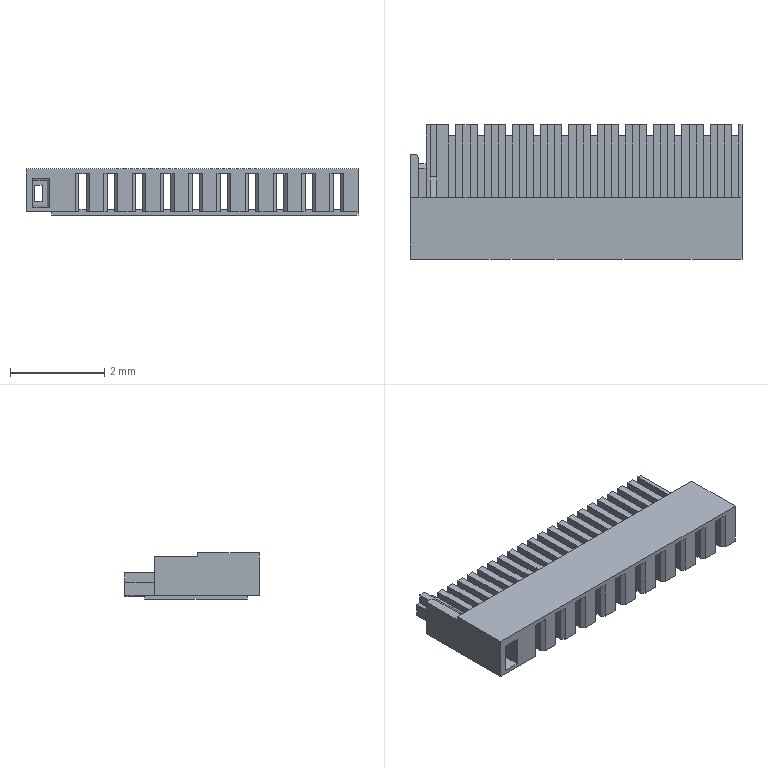Part | Creo | 1 solid | 312 faces | box 7.05 x 2.85 x 0.98 mm | volume 7.612 mm3 | plane 312